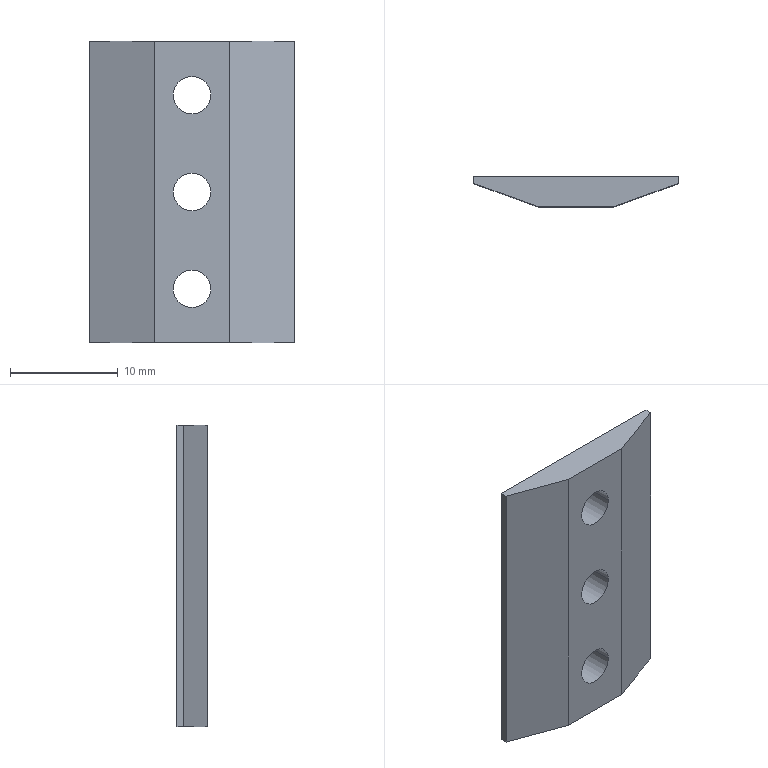Part | NX | 1 solid | 14 faces | box 19 x 2.8 x 28 mm | volume 1042 mm3 | plane 8 | cylinder 6 | commonest cylinder face diameters 3.5 x6
STEP:
#1=CARTESIAN_POINT('',(19.,2.8,0.));
#2=VERTEX_POINT('',#1);
#3=CARTESIAN_POINT('',(0.,2.8,0.));
#4=VERTEX_POINT('',#3);
#5=CARTESIAN_POINT('',(0.,2.8,0.));
#6=DIRECTION('',(-1.,0.,0.));
#7=VECTOR('',#6,1000.);
#8=LINE('',#5,#7);
#9=EDGE_CURVE('',#2,#4,#8,.T.);
#10=ORIENTED_EDGE('',*,*,#9,.F.);
#11=CARTESIAN_POINT('',(19.,2.8,-28.));
#12=VERTEX_POINT('',#11);
#13=CARTESIAN_POINT('',(19.,2.8,0.));
#14=DIRECTION('',(0.,0.,1.));
#15=VECTOR('',#14,1000.);
#16=LINE('',#13,#15);
#17=EDGE_CURVE('',#12,#2,#16,.T.);
#18=ORIENTED_EDGE('',*,*,#17,.F.);
#19=CARTESIAN_POINT('',(0.,2.8,-28.));
#20=VERTEX_POINT('',#19);
#21=CARTESIAN_POINT('',(0.,2.8,-28.));
#22=DIRECTION('',(1.,0.,0.));
#23=VECTOR('',#22,1000.);
#24=LINE('',#21,#23);
#25=EDGE_CURVE('',#20,#12,#24,.T.);
#26=ORIENTED_EDGE('',*,*,#25,.F.);
#27=CARTESIAN_POINT('',(0.,2.8,0.));
#28=DIRECTION('',(0.,0.,-1.));
#29=VECTOR('',#28,1000.);
#30=LINE('',#27,#29);
#31=EDGE_CURVE('',#4,#20,#30,.T.);
#32=ORIENTED_EDGE('',*,*,#31,.F.);
#33=EDGE_LOOP('',(#10,#18,#26,#32));
#34=FACE_BOUND('',#33,.T.);
#35=CARTESIAN_POINT('',(11.25,2.8,-23.));
#36=VERTEX_POINT('',#35);
#37=CARTESIAN_POINT('',(7.75,2.8,-23.));
#38=VERTEX_POINT('',#37);
#39=CARTESIAN_POINT('',(9.5,2.8,-23.));
#40=DIRECTION('',(0.,-1.,0.));
#41=DIRECTION('',(1.,0.,0.));
#42=AXIS2_PLACEMENT_3D('',#39,#40,#41);
#43=CIRCLE('',#42,1.75);
#44=EDGE_CURVE('',#36,#38,#43,.T.);
#45=ORIENTED_EDGE('',*,*,#44,.T.);
#46=CARTESIAN_POINT('',(9.5,2.8,-23.));
#47=DIRECTION('',(0.,-1.,0.));
#48=DIRECTION('',(1.,0.,0.));
#49=AXIS2_PLACEMENT_3D('',#46,#47,#48);
#50=CIRCLE('',#49,1.75);
#51=EDGE_CURVE('',#38,#36,#50,.T.);
#52=ORIENTED_EDGE('',*,*,#51,.T.);
#53=EDGE_LOOP('',(#45,#52));
#54=FACE_BOUND('',#53,.T.);
#55=CARTESIAN_POINT('',(11.25,2.8,-14.));
#56=VERTEX_POINT('',#55);
#57=CARTESIAN_POINT('',(7.75,2.8,-14.));
#58=VERTEX_POINT('',#57);
#59=CARTESIAN_POINT('',(9.5,2.8,-14.));
#60=DIRECTION('',(0.,-1.,0.));
#61=DIRECTION('',(1.,0.,0.));
#62=AXIS2_PLACEMENT_3D('',#59,#60,#61);
#63=CIRCLE('',#62,1.75);
#64=EDGE_CURVE('',#56,#58,#63,.T.);
#65=ORIENTED_EDGE('',*,*,#64,.T.);
#66=CARTESIAN_POINT('',(9.5,2.8,-14.));
#67=DIRECTION('',(0.,-1.,0.));
#68=DIRECTION('',(1.,0.,0.));
#69=AXIS2_PLACEMENT_3D('',#66,#67,#68);
#70=CIRCLE('',#69,1.75);
#71=EDGE_CURVE('',#58,#56,#70,.T.);
#72=ORIENTED_EDGE('',*,*,#71,.T.);
#73=EDGE_LOOP('',(#65,#72));
#74=FACE_BOUND('',#73,.T.);
#75=CARTESIAN_POINT('',(11.25,2.8,-5.));
#76=VERTEX_POINT('',#75);
#77=CARTESIAN_POINT('',(7.75,2.8,-5.));
#78=VERTEX_POINT('',#77);
#79=CARTESIAN_POINT('',(9.5,2.8,-5.));
#80=DIRECTION('',(0.,-1.,0.));
#81=DIRECTION('',(1.,0.,0.));
#82=AXIS2_PLACEMENT_3D('',#79,#80,#81);
#83=CIRCLE('',#82,1.75);
#84=EDGE_CURVE('',#76,#78,#83,.T.);
#85=ORIENTED_EDGE('',*,*,#84,.T.);
#86=CARTESIAN_POINT('',(9.5,2.8,-5.));
#87=DIRECTION('',(0.,-1.,0.));
#88=DIRECTION('',(1.,0.,0.));
#89=AXIS2_PLACEMENT_3D('',#86,#87,#88);
#90=CIRCLE('',#89,1.75);
#91=EDGE_CURVE('',#78,#76,#90,.T.);
#92=ORIENTED_EDGE('',*,*,#91,.T.);
#93=EDGE_LOOP('',(#85,#92));
#94=FACE_BOUND('',#93,.T.);
#95=CARTESIAN_POINT('',(0.,2.8,0.));
#96=DIRECTION('',(0.,1.,0.));
#97=DIRECTION('',(1.,0.,0.));
#98=AXIS2_PLACEMENT_3D('',#95,#96,#97);
#99=PLANE('',#98);
#100=ADVANCED_FACE('',(#34,#54,#74,#94),#99,.T.);
#101=CARTESIAN_POINT('',(13.,0.,0.));
#102=VERTEX_POINT('',#101);
#103=CARTESIAN_POINT('',(6.,0.,0.));
#104=VERTEX_POINT('',#103);
#105=CARTESIAN_POINT('',(0.,0.,0.));
#106=DIRECTION('',(-1.,0.,0.));
#107=VECTOR('',#106,1000.);
#108=LINE('',#105,#107);
#109=EDGE_CURVE('',#102,#104,#108,.T.);
#110=ORIENTED_EDGE('',*,*,#109,.F.);
#111=CARTESIAN_POINT('',(19.,2.184,0.));
#112=VERTEX_POINT('',#111);
#113=CARTESIAN_POINT('',(13.,0.,0.));
#114=CARTESIAN_POINT('',(15.,0.7279,0.));
#115=CARTESIAN_POINT('',(17.,1.456,0.));
#116=CARTESIAN_POINT('',(19.,2.184,0.));
#117=B_SPLINE_CURVE_WITH_KNOTS('',3,(#113,#114,#115,#116),.UNSPECIFIED.,.F.,.F.,(4,4),(0.,1.),.UNSPECIFIED.);
#118=EDGE_CURVE('',#112,#102,#117,.F.);
#119=ORIENTED_EDGE('',*,*,#118,.F.);
#120=CARTESIAN_POINT('',(19.,2.184,0.));
#121=CARTESIAN_POINT('',(19.,2.389,0.));
#122=CARTESIAN_POINT('',(19.,2.595,0.));
#123=CARTESIAN_POINT('',(19.,2.8,0.));
#124=B_SPLINE_CURVE_WITH_KNOTS('',3,(#120,#121,#122,#123),.UNSPECIFIED.,.F.,.F.,(4,4),(0.,1.),.UNSPECIFIED.);
#125=EDGE_CURVE('',#2,#112,#124,.F.);
#126=ORIENTED_EDGE('',*,*,#125,.F.);
#127=ORIENTED_EDGE('',*,*,#9,.T.);
#128=CARTESIAN_POINT('',(0.,2.184,0.));
#129=VERTEX_POINT('',#128);
#130=CARTESIAN_POINT('',(0.,2.8,0.));
#131=DIRECTION('',(0.,-1.,0.));
#132=VECTOR('',#131,1000.);
#133=LINE('',#130,#132);
#134=EDGE_CURVE('',#4,#129,#133,.T.);
#135=ORIENTED_EDGE('',*,*,#134,.T.);
#136=CARTESIAN_POINT('',(6.,0.,0.));
#137=DIRECTION('',(-0.9397,0.342,0.));
#138=VECTOR('',#137,1000.);
#139=LINE('',#136,#138);
#140=EDGE_CURVE('',#104,#129,#139,.T.);
#141=ORIENTED_EDGE('',*,*,#140,.F.);
#142=EDGE_LOOP('',(#110,#119,#126,#127,#135,#141));
#143=FACE_BOUND('',#142,.T.);
#144=CARTESIAN_POINT('',(0.,0.,0.));
#145=DIRECTION('',(0.,0.,1.));
#146=DIRECTION('',(1.,0.,0.));
#147=AXIS2_PLACEMENT_3D('',#144,#145,#146);
#148=PLANE('',#147);
#149=ADVANCED_FACE('',(#143),#148,.T.);
#150=CARTESIAN_POINT('',(6.,0.,-28.));
#151=VERTEX_POINT('',#150);
#152=CARTESIAN_POINT('',(6.,0.,0.));
#153=DIRECTION('',(0.,0.,-1.));
#154=VECTOR('',#153,1000.);
#155=LINE('',#152,#154);
#156=EDGE_CURVE('',#104,#151,#155,.T.);
#157=ORIENTED_EDGE('',*,*,#156,.F.);
#158=ORIENTED_EDGE('',*,*,#140,.T.);
#159=CARTESIAN_POINT('',(0.,2.184,-28.));
#160=VERTEX_POINT('',#159);
#161=CARTESIAN_POINT('',(0.,2.184,0.));
#162=DIRECTION('',(0.,0.,-1.));
#163=VECTOR('',#162,1000.);
#164=LINE('',#161,#163);
#165=EDGE_CURVE('',#129,#160,#164,.T.);
#166=ORIENTED_EDGE('',*,*,#165,.T.);
#167=CARTESIAN_POINT('',(0.,2.184,-28.));
#168=DIRECTION('',(0.9397,-0.342,0.));
#169=VECTOR('',#168,1000.);
#170=LINE('',#167,#169);
#171=EDGE_CURVE('',#160,#151,#170,.T.);
#172=ORIENTED_EDGE('',*,*,#171,.T.);
#173=EDGE_LOOP('',(#157,#158,#166,#172));
#174=FACE_BOUND('',#173,.T.);
#175=CARTESIAN_POINT('',(6.,0.,-28.));
#176=DIRECTION('',(-0.342,-0.9397,0.));
#177=DIRECTION('',(-0.9397,0.342,0.));
#178=AXIS2_PLACEMENT_3D('',#175,#176,#177);
#179=PLANE('',#178);
#180=ADVANCED_FACE('',(#174),#179,.T.);
#181=CARTESIAN_POINT('',(13.,0.,-28.));
#182=VERTEX_POINT('',#181);
#183=CARTESIAN_POINT('',(0.,0.,-28.));
#184=DIRECTION('',(1.,0.,0.));
#185=VECTOR('',#184,1000.);
#186=LINE('',#183,#185);
#187=EDGE_CURVE('',#151,#182,#186,.T.);
#188=ORIENTED_EDGE('',*,*,#187,.F.);
#189=ORIENTED_EDGE('',*,*,#171,.F.);
#190=CARTESIAN_POINT('',(0.,2.8,-28.));
#191=DIRECTION('',(0.,-1.,0.));
#192=VECTOR('',#191,1000.);
#193=LINE('',#190,#192);
#194=EDGE_CURVE('',#20,#160,#193,.T.);
#195=ORIENTED_EDGE('',*,*,#194,.F.);
#196=ORIENTED_EDGE('',*,*,#25,.T.);
#197=CARTESIAN_POINT('',(19.,2.184,-28.));
#198=VERTEX_POINT('',#197);
#199=CARTESIAN_POINT('',(19.,2.8,-28.));
#200=CARTESIAN_POINT('',(19.,2.595,-28.));
#201=CARTESIAN_POINT('',(19.,2.389,-28.));
#202=CARTESIAN_POINT('',(19.,2.184,-28.));
#203=B_SPLINE_CURVE_WITH_KNOTS('',3,(#199,#200,#201,#202),.UNSPECIFIED.,.F.,.F.,(4,4),(0.,1.),.UNSPECIFIED.);
#204=EDGE_CURVE('',#12,#198,#203,.T.);
#205=ORIENTED_EDGE('',*,*,#204,.T.);
#206=CARTESIAN_POINT('',(19.,2.184,-28.));
#207=CARTESIAN_POINT('',(17.,1.456,-28.));
#208=CARTESIAN_POINT('',(15.,0.7279,-28.));
#209=CARTESIAN_POINT('',(13.,0.,-28.));
#210=B_SPLINE_CURVE_WITH_KNOTS('',3,(#206,#207,#208,#209),.UNSPECIFIED.,.F.,.F.,(4,4),(0.,1.),.UNSPECIFIED.);
#211=EDGE_CURVE('',#182,#198,#210,.F.);
#212=ORIENTED_EDGE('',*,*,#211,.F.);
#213=EDGE_LOOP('',(#188,#189,#195,#196,#205,#212));
#214=FACE_BOUND('',#213,.T.);
#215=CARTESIAN_POINT('',(19.,0.,-28.));
#216=DIRECTION('',(0.,0.,-1.));
#217=DIRECTION('',(0.,-1.,0.));
#218=AXIS2_PLACEMENT_3D('',#215,#216,#217);
#219=PLANE('',#218);
#220=ADVANCED_FACE('',(#214),#219,.T.);
#221=CARTESIAN_POINT('',(13.,0.,0.));
#222=DIRECTION('',(0.,0.,1.));
#223=VECTOR('',#222,1000.);
#224=LINE('',#221,#223);
#225=EDGE_CURVE('',#182,#102,#224,.T.);
#226=ORIENTED_EDGE('',*,*,#225,.F.);
#227=ORIENTED_EDGE('',*,*,#211,.T.);
#228=CARTESIAN_POINT('',(19.,2.184,-28.));
#229=CARTESIAN_POINT('',(19.,2.184,-18.667));
#230=CARTESIAN_POINT('',(19.,2.184,-9.333));
#231=CARTESIAN_POINT('',(19.,2.184,0.));
#232=B_SPLINE_CURVE_WITH_KNOTS('',3,(#228,#229,#230,#231),.UNSPECIFIED.,.F.,.F.,(4,4),(0.,1.),.UNSPECIFIED.);
#233=EDGE_CURVE('',#198,#112,#232,.T.);
#234=ORIENTED_EDGE('',*,*,#233,.T.);
#235=ORIENTED_EDGE('',*,*,#118,.T.);
#236=EDGE_LOOP('',(#226,#227,#234,#235));
#237=FACE_BOUND('',#236,.T.);
#238=CARTESIAN_POINT('',(13.,0.,0.));
#239=DIRECTION('',(0.342,-0.9397,0.));
#240=DIRECTION('',(0.,0.,-1.));
#241=AXIS2_PLACEMENT_3D('',#238,#239,#240);
#242=PLANE('',#241);
#243=ADVANCED_FACE('',(#237),#242,.T.);
#244=ORIENTED_EDGE('',*,*,#233,.F.);
#245=ORIENTED_EDGE('',*,*,#204,.F.);
#246=ORIENTED_EDGE('',*,*,#17,.T.);
#247=ORIENTED_EDGE('',*,*,#125,.T.);
#248=EDGE_LOOP('',(#244,#245,#246,#247));
#249=FACE_BOUND('',#248,.T.);
#250=CARTESIAN_POINT('',(19.,0.,0.));
#251=DIRECTION('',(1.,0.,0.));
#252=DIRECTION('',(0.,1.,0.));
#253=AXIS2_PLACEMENT_3D('',#250,#251,#252);
#254=PLANE('',#253);
#255=ADVANCED_FACE('',(#249),#254,.T.);
#256=ORIENTED_EDGE('',*,*,#109,.T.);
#257=ORIENTED_EDGE('',*,*,#156,.T.);
#258=ORIENTED_EDGE('',*,*,#187,.T.);
#259=ORIENTED_EDGE('',*,*,#225,.T.);
#260=EDGE_LOOP('',(#256,#257,#258,#259));
#261=FACE_BOUND('',#260,.T.);
#262=CARTESIAN_POINT('',(7.75,0.,-23.));
#263=VERTEX_POINT('',#262);
#264=CARTESIAN_POINT('',(11.25,0.,-23.));
#265=VERTEX_POINT('',#264);
#266=CARTESIAN_POINT('',(9.5,0.,-23.));
#267=DIRECTION('',(0.,-1.,0.));
#268=DIRECTION('',(1.,0.,0.));
#269=AXIS2_PLACEMENT_3D('',#266,#267,#268);
#270=CIRCLE('',#269,1.75);
#271=EDGE_CURVE('',#263,#265,#270,.T.);
#272=ORIENTED_EDGE('',*,*,#271,.F.);
#273=CARTESIAN_POINT('',(9.5,0.,-23.));
#274=DIRECTION('',(0.,-1.,0.));
#275=DIRECTION('',(1.,0.,0.));
#276=AXIS2_PLACEMENT_3D('',#273,#274,#275);
#277=CIRCLE('',#276,1.75);
#278=EDGE_CURVE('',#265,#263,#277,.T.);
#279=ORIENTED_EDGE('',*,*,#278,.F.);
#280=EDGE_LOOP('',(#272,#279));
#281=FACE_BOUND('',#280,.T.);
#282=CARTESIAN_POINT('',(7.75,0.,-14.));
#283=VERTEX_POINT('',#282);
#284=CARTESIAN_POINT('',(11.25,0.,-14.));
#285=VERTEX_POINT('',#284);
#286=CARTESIAN_POINT('',(9.5,0.,-14.));
#287=DIRECTION('',(0.,-1.,0.));
#288=DIRECTION('',(1.,0.,0.));
#289=AXIS2_PLACEMENT_3D('',#286,#287,#288);
#290=CIRCLE('',#289,1.75);
#291=EDGE_CURVE('',#283,#285,#290,.T.);
#292=ORIENTED_EDGE('',*,*,#291,.F.);
#293=CARTESIAN_POINT('',(9.5,0.,-14.));
#294=DIRECTION('',(0.,-1.,0.));
#295=DIRECTION('',(1.,0.,0.));
#296=AXIS2_PLACEMENT_3D('',#293,#294,#295);
#297=CIRCLE('',#296,1.75);
#298=EDGE_CURVE('',#285,#283,#297,.T.);
#299=ORIENTED_EDGE('',*,*,#298,.F.);
#300=EDGE_LOOP('',(#292,#299));
#301=FACE_BOUND('',#300,.T.);
#302=CARTESIAN_POINT('',(7.75,0.,-5.));
#303=VERTEX_POINT('',#302);
#304=CARTESIAN_POINT('',(11.25,0.,-5.));
#305=VERTEX_POINT('',#304);
#306=CARTESIAN_POINT('',(9.5,0.,-5.));
#307=DIRECTION('',(0.,-1.,0.));
#308=DIRECTION('',(1.,0.,0.));
#309=AXIS2_PLACEMENT_3D('',#306,#307,#308);
#310=CIRCLE('',#309,1.75);
#311=EDGE_CURVE('',#303,#305,#310,.T.);
#312=ORIENTED_EDGE('',*,*,#311,.F.);
#313=CARTESIAN_POINT('',(9.5,0.,-5.));
#314=DIRECTION('',(0.,-1.,0.));
#315=DIRECTION('',(1.,0.,0.));
#316=AXIS2_PLACEMENT_3D('',#313,#314,#315);
#317=CIRCLE('',#316,1.75);
#318=EDGE_CURVE('',#305,#303,#317,.T.);
#319=ORIENTED_EDGE('',*,*,#318,.F.);
#320=EDGE_LOOP('',(#312,#319));
#321=FACE_BOUND('',#320,.T.);
#322=CARTESIAN_POINT('',(0.,0.,0.));
#323=DIRECTION('',(0.,1.,0.));
#324=DIRECTION('',(1.,0.,0.));
#325=AXIS2_PLACEMENT_3D('',#322,#323,#324);
#326=PLANE('',#325);
#327=ADVANCED_FACE('',(#261,#281,#301,#321),#326,.F.);
#328=ORIENTED_EDGE('',*,*,#165,.F.);
#329=ORIENTED_EDGE('',*,*,#134,.F.);
#330=ORIENTED_EDGE('',*,*,#31,.T.);
#331=ORIENTED_EDGE('',*,*,#194,.T.);
#332=EDGE_LOOP('',(#328,#329,#330,#331));
#333=FACE_BOUND('',#332,.T.);
#334=CARTESIAN_POINT('',(0.,0.,-28.));
#335=DIRECTION('',(-1.,0.,0.));
#336=DIRECTION('',(0.,0.,1.));
#337=AXIS2_PLACEMENT_3D('',#334,#335,#336);
#338=PLANE('',#337);
#339=ADVANCED_FACE('',(#333),#338,.T.);
#340=ORIENTED_EDGE('',*,*,#271,.T.);
#341=CARTESIAN_POINT('',(11.25,2.8,-23.));
#342=DIRECTION('',(0.,-1.,0.));
#343=VECTOR('',#342,1000.);
#344=LINE('',#341,#343);
#345=EDGE_CURVE('',#36,#265,#344,.T.);
#346=ORIENTED_EDGE('',*,*,#345,.F.);
#347=ORIENTED_EDGE('',*,*,#51,.F.);
#348=CARTESIAN_POINT('',(7.75,2.8,-23.));
#349=DIRECTION('',(0.,-1.,0.));
#350=VECTOR('',#349,1000.);
#351=LINE('',#348,#350);
#352=EDGE_CURVE('',#38,#263,#351,.T.);
#353=ORIENTED_EDGE('',*,*,#352,.T.);
#354=EDGE_LOOP('',(#340,#346,#347,#353));
#355=FACE_BOUND('',#354,.T.);
#356=CARTESIAN_POINT('',(9.5,2.8,-23.));
#357=DIRECTION('',(0.,-1.,0.));
#358=DIRECTION('',(1.,0.,0.));
#359=AXIS2_PLACEMENT_3D('',#356,#357,#358);
#360=CYLINDRICAL_SURFACE('',#359,1.75);
#361=ADVANCED_FACE('',(#355),#360,.F.);
#362=ORIENTED_EDGE('',*,*,#64,.F.);
#363=CARTESIAN_POINT('',(11.25,2.8,-14.));
#364=DIRECTION('',(0.,-1.,0.));
#365=VECTOR('',#364,1000.);
#366=LINE('',#363,#365);
#367=EDGE_CURVE('',#56,#285,#366,.T.);
#368=ORIENTED_EDGE('',*,*,#367,.T.);
#369=ORIENTED_EDGE('',*,*,#298,.T.);
#370=CARTESIAN_POINT('',(7.75,2.8,-14.));
#371=DIRECTION('',(0.,-1.,0.));
#372=VECTOR('',#371,1000.);
#373=LINE('',#370,#372);
#374=EDGE_CURVE('',#58,#283,#373,.T.);
#375=ORIENTED_EDGE('',*,*,#374,.F.);
#376=EDGE_LOOP('',(#362,#368,#369,#375));
#377=FACE_BOUND('',#376,.T.);
#378=CARTESIAN_POINT('',(9.5,2.8,-14.));
#379=DIRECTION('',(0.,-1.,0.));
#380=DIRECTION('',(1.,0.,0.));
#381=AXIS2_PLACEMENT_3D('',#378,#379,#380);
#382=CYLINDRICAL_SURFACE('',#381,1.75);
#383=ADVANCED_FACE('',(#377),#382,.F.);
#384=ORIENTED_EDGE('',*,*,#84,.F.);
#385=CARTESIAN_POINT('',(11.25,2.8,-5.));
#386=DIRECTION('',(0.,-1.,0.));
#387=VECTOR('',#386,1000.);
#388=LINE('',#385,#387);
#389=EDGE_CURVE('',#76,#305,#388,.T.);
#390=ORIENTED_EDGE('',*,*,#389,.T.);
#391=ORIENTED_EDGE('',*,*,#318,.T.);
#392=CARTESIAN_POINT('',(7.75,2.8,-5.));
#393=DIRECTION('',(0.,-1.,0.));
#394=VECTOR('',#393,1000.);
#395=LINE('',#392,#394);
#396=EDGE_CURVE('',#78,#303,#395,.T.);
#397=ORIENTED_EDGE('',*,*,#396,.F.);
#398=EDGE_LOOP('',(#384,#390,#391,#397));
#399=FACE_BOUND('',#398,.T.);
#400=CARTESIAN_POINT('',(9.5,2.8,-5.));
#401=DIRECTION('',(0.,-1.,0.));
#402=DIRECTION('',(1.,0.,0.));
#403=AXIS2_PLACEMENT_3D('',#400,#401,#402);
#404=CYLINDRICAL_SURFACE('',#403,1.75);
#405=ADVANCED_FACE('',(#399),#404,.F.);
#406=ORIENTED_EDGE('',*,*,#311,.T.);
#407=ORIENTED_EDGE('',*,*,#389,.F.);
#408=ORIENTED_EDGE('',*,*,#91,.F.);
#409=ORIENTED_EDGE('',*,*,#396,.T.);
#410=EDGE_LOOP('',(#406,#407,#408,#409));
#411=FACE_BOUND('',#410,.T.);
#412=CARTESIAN_POINT('',(9.5,2.8,-5.));
#413=DIRECTION('',(0.,-1.,0.));
#414=DIRECTION('',(1.,0.,0.));
#415=AXIS2_PLACEMENT_3D('',#412,#413,#414);
#416=CYLINDRICAL_SURFACE('',#415,1.75);
#417=ADVANCED_FACE('',(#411),#416,.F.);
#418=ORIENTED_EDGE('',*,*,#291,.T.);
#419=ORIENTED_EDGE('',*,*,#367,.F.);
#420=ORIENTED_EDGE('',*,*,#71,.F.);
#421=ORIENTED_EDGE('',*,*,#374,.T.);
#422=EDGE_LOOP('',(#418,#419,#420,#421));
#423=FACE_BOUND('',#422,.T.);
#424=CARTESIAN_POINT('',(9.5,2.8,-14.));
#425=DIRECTION('',(0.,-1.,0.));
#426=DIRECTION('',(1.,0.,0.));
#427=AXIS2_PLACEMENT_3D('',#424,#425,#426);
#428=CYLINDRICAL_SURFACE('',#427,1.75);
#429=ADVANCED_FACE('',(#423),#428,.F.);
#430=ORIENTED_EDGE('',*,*,#44,.F.);
#431=ORIENTED_EDGE('',*,*,#345,.T.);
#432=ORIENTED_EDGE('',*,*,#278,.T.);
#433=ORIENTED_EDGE('',*,*,#352,.F.);
#434=EDGE_LOOP('',(#430,#431,#432,#433));
#435=FACE_BOUND('',#434,.T.);
#436=CARTESIAN_POINT('',(9.5,2.8,-23.));
#437=DIRECTION('',(0.,-1.,0.));
#438=DIRECTION('',(1.,0.,0.));
#439=AXIS2_PLACEMENT_3D('',#436,#437,#438);
#440=CYLINDRICAL_SURFACE('',#439,1.75);
#441=ADVANCED_FACE('',(#435),#440,.F.);
#442=CLOSED_SHELL('',(#100,#149,#180,#220,#243,#255,#327,#339,#361,#383,#405,#417,#429,#441));
#443=MANIFOLD_SOLID_BREP('',#442);
#444=(LENGTH_UNIT()NAMED_UNIT(*)SI_UNIT(.MILLI.,.METRE.));
#445=UNCERTAINTY_MEASURE_WITH_UNIT(LENGTH_MEASURE(0.0508),#444,'','');
#446=(NAMED_UNIT(*)PLANE_ANGLE_UNIT()SI_UNIT($,.RADIAN.));
#447=(NAMED_UNIT(*)SI_UNIT($,.STERADIAN.)SOLID_ANGLE_UNIT());
#448=(GEOMETRIC_REPRESENTATION_CONTEXT(3)GLOBAL_UNCERTAINTY_ASSIGNED_CONTEXT((#445))GLOBAL_UNIT_ASSIGNED_CONTEXT((#444,#446,#447))REPRESENTATION_CONTEXT('',''));
#449=ADVANCED_BREP_SHAPE_REPRESENTATION('',(#443),#448);